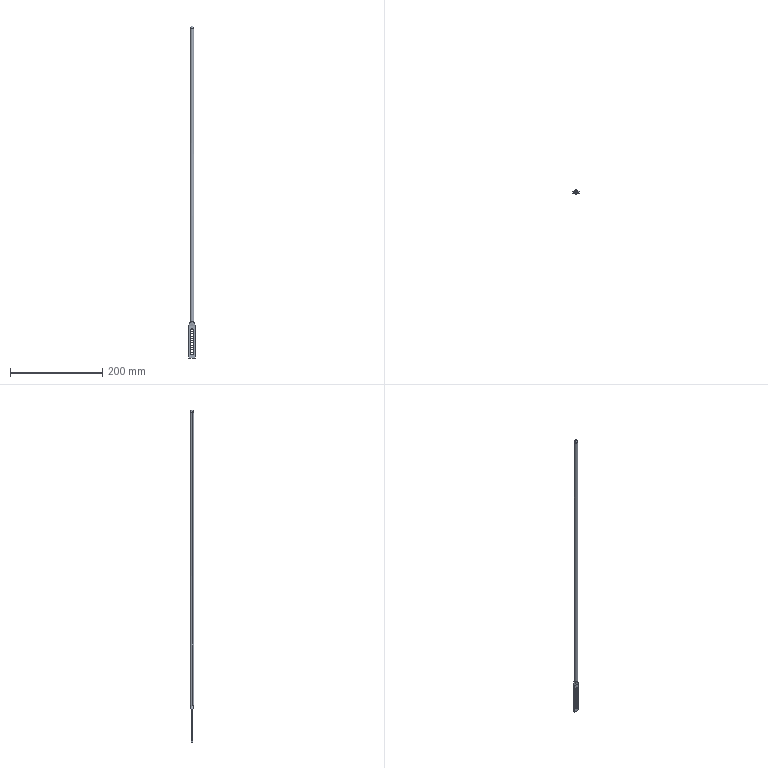Part | STEP file | _X2_751F4E45_X0_LG003_X2_8-1051 | 1 solid | 34 faces | box 14 x 8.003 x 719 mm | volume 34906 mm3 | cylinder 22 | plane 6 | spline 4 | cone 2 | commonest cylinder face diameters 6.1 x20 8 x2